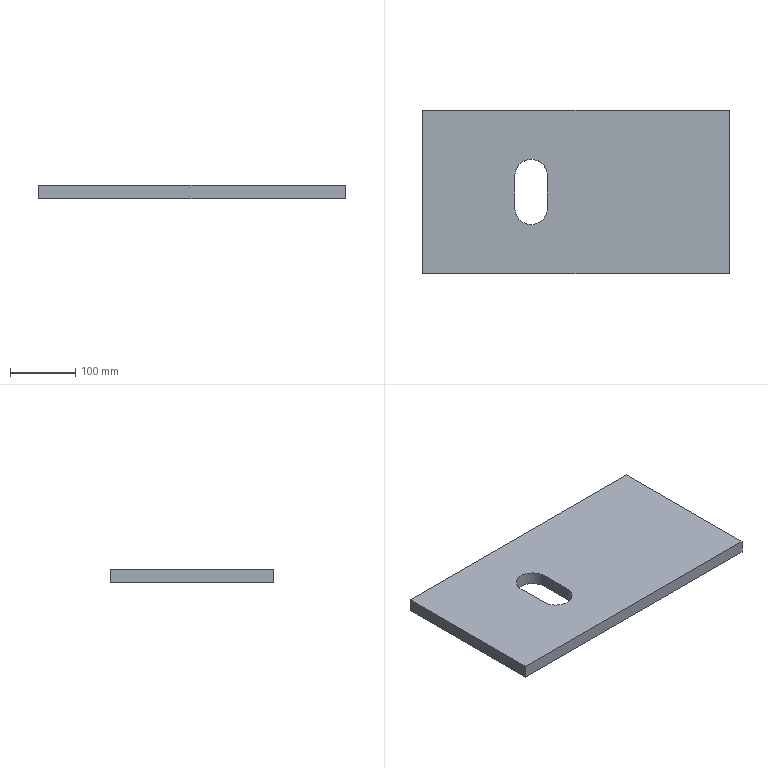Part | SolidWorks | features Extrusion 1 | 1 solid | 12 faces | box 468.5 x 250 x 20 mm | volume 2253231 mm3 | plane 8 | cylinder 4 | commonest cylinder face diameters 50 x4